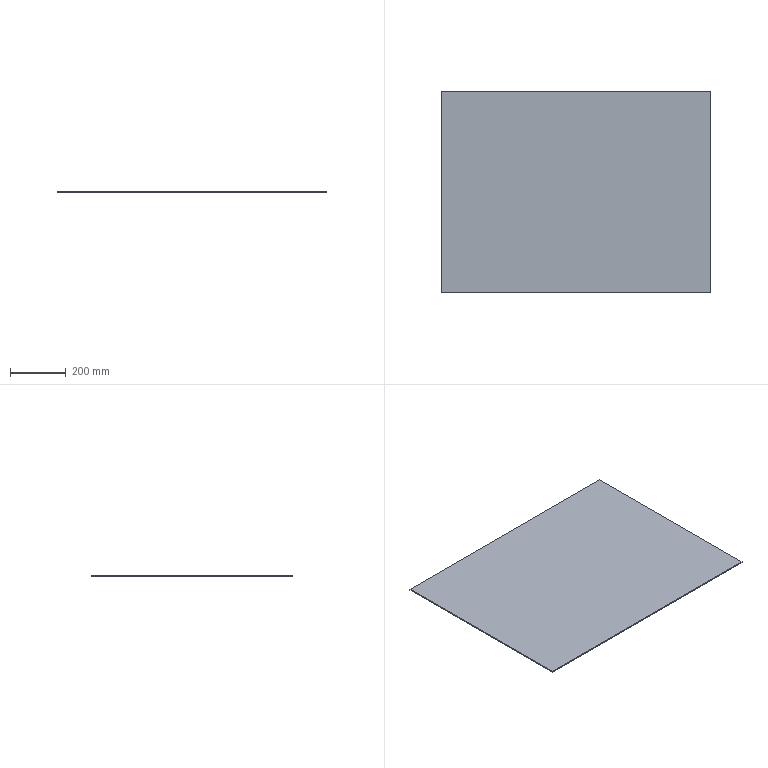Part | STEP file | X77-05501 | 1 solid | 6 faces | box 960 x 720 x 4 mm | volume 2764800 mm3 | plane 6
STEP:
#1=CARTESIAN_POINT('',(521.386,-150.547,0.));
#2=VERTEX_POINT('',#1);
#3=CARTESIAN_POINT('',(521.386,-870.547,0.));
#4=VERTEX_POINT('',#3);
#5=CARTESIAN_POINT('',(521.386,-870.547,0.));
#6=DIRECTION('',(0.,-1.,0.));
#7=VECTOR('',#6,1000.);
#8=LINE('',#5,#7);
#9=EDGE_CURVE('',#2,#4,#8,.T.);
#10=ORIENTED_EDGE('',*,*,#9,.T.);
#11=CARTESIAN_POINT('',(521.386,-870.547,4.));
#12=VERTEX_POINT('',#11);
#13=CARTESIAN_POINT('',(521.386,-870.547,4.));
#14=DIRECTION('',(0.,0.,-1.));
#15=VECTOR('',#14,1000.);
#16=LINE('',#13,#15);
#17=EDGE_CURVE('',#12,#4,#16,.T.);
#18=ORIENTED_EDGE('',*,*,#17,.F.);
#19=CARTESIAN_POINT('',(521.386,-150.547,4.));
#20=VERTEX_POINT('',#19);
#21=CARTESIAN_POINT('',(521.386,-870.547,4.));
#22=DIRECTION('',(0.,-1.,0.));
#23=VECTOR('',#22,1000.);
#24=LINE('',#21,#23);
#25=EDGE_CURVE('',#20,#12,#24,.T.);
#26=ORIENTED_EDGE('',*,*,#25,.F.);
#27=CARTESIAN_POINT('',(521.386,-150.547,4.));
#28=DIRECTION('',(0.,0.,-1.));
#29=VECTOR('',#28,1000.);
#30=LINE('',#27,#29);
#31=EDGE_CURVE('',#20,#2,#30,.T.);
#32=ORIENTED_EDGE('',*,*,#31,.T.);
#33=EDGE_LOOP('',(#10,#18,#26,#32));
#34=FACE_OUTER_BOUND('',#33,.T.);
#35=CARTESIAN_POINT('',(521.386,-870.547,4.));
#36=DIRECTION('',(1.,0.,0.));
#37=DIRECTION('',(0.,0.,-1.));
#38=AXIS2_PLACEMENT_3D('',#35,#36,#37);
#39=PLANE('',#38);
#40=ADVANCED_FACE('',(#34),#39,.F.);
#41=CARTESIAN_POINT('',(1481.386,-870.547,0.));
#42=VERTEX_POINT('',#41);
#43=CARTESIAN_POINT('',(521.386,-870.547,0.));
#44=DIRECTION('',(1.,0.,0.));
#45=VECTOR('',#44,1000.);
#46=LINE('',#43,#45);
#47=EDGE_CURVE('',#4,#42,#46,.T.);
#48=ORIENTED_EDGE('',*,*,#47,.T.);
#49=CARTESIAN_POINT('',(1481.386,-870.547,4.));
#50=VERTEX_POINT('',#49);
#51=CARTESIAN_POINT('',(1481.386,-870.547,4.));
#52=DIRECTION('',(0.,0.,-1.));
#53=VECTOR('',#52,1000.);
#54=LINE('',#51,#53);
#55=EDGE_CURVE('',#50,#42,#54,.T.);
#56=ORIENTED_EDGE('',*,*,#55,.F.);
#57=CARTESIAN_POINT('',(521.386,-870.547,4.));
#58=DIRECTION('',(1.,0.,0.));
#59=VECTOR('',#58,1000.);
#60=LINE('',#57,#59);
#61=EDGE_CURVE('',#12,#50,#60,.T.);
#62=ORIENTED_EDGE('',*,*,#61,.F.);
#63=ORIENTED_EDGE('',*,*,#17,.T.);
#64=EDGE_LOOP('',(#48,#56,#62,#63));
#65=FACE_OUTER_BOUND('',#64,.T.);
#66=CARTESIAN_POINT('',(521.386,-870.547,4.));
#67=DIRECTION('',(0.,1.,0.));
#68=DIRECTION('',(0.,0.,1.));
#69=AXIS2_PLACEMENT_3D('',#66,#67,#68);
#70=PLANE('',#69);
#71=ADVANCED_FACE('',(#65),#70,.F.);
#72=CARTESIAN_POINT('',(1481.386,-150.547,0.));
#73=VERTEX_POINT('',#72);
#74=CARTESIAN_POINT('',(1481.386,-870.547,0.));
#75=DIRECTION('',(0.,1.,0.));
#76=VECTOR('',#75,1000.);
#77=LINE('',#74,#76);
#78=EDGE_CURVE('',#42,#73,#77,.T.);
#79=ORIENTED_EDGE('',*,*,#78,.T.);
#80=CARTESIAN_POINT('',(1481.386,-150.547,4.));
#81=VERTEX_POINT('',#80);
#82=CARTESIAN_POINT('',(1481.386,-150.547,4.));
#83=DIRECTION('',(0.,0.,-1.));
#84=VECTOR('',#83,1000.);
#85=LINE('',#82,#84);
#86=EDGE_CURVE('',#81,#73,#85,.T.);
#87=ORIENTED_EDGE('',*,*,#86,.F.);
#88=CARTESIAN_POINT('',(1481.386,-870.547,4.));
#89=DIRECTION('',(0.,1.,0.));
#90=VECTOR('',#89,1000.);
#91=LINE('',#88,#90);
#92=EDGE_CURVE('',#50,#81,#91,.T.);
#93=ORIENTED_EDGE('',*,*,#92,.F.);
#94=ORIENTED_EDGE('',*,*,#55,.T.);
#95=EDGE_LOOP('',(#79,#87,#93,#94));
#96=FACE_OUTER_BOUND('',#95,.T.);
#97=CARTESIAN_POINT('',(1481.386,-870.547,4.));
#98=DIRECTION('',(-1.,0.,0.));
#99=DIRECTION('',(0.,0.,1.));
#100=AXIS2_PLACEMENT_3D('',#97,#98,#99);
#101=PLANE('',#100);
#102=ADVANCED_FACE('',(#96),#101,.F.);
#103=CARTESIAN_POINT('',(521.386,-150.547,0.));
#104=DIRECTION('',(-1.,0.,0.));
#105=VECTOR('',#104,1000.);
#106=LINE('',#103,#105);
#107=EDGE_CURVE('',#73,#2,#106,.T.);
#108=ORIENTED_EDGE('',*,*,#107,.T.);
#109=ORIENTED_EDGE('',*,*,#31,.F.);
#110=CARTESIAN_POINT('',(521.386,-150.547,4.));
#111=DIRECTION('',(-1.,0.,0.));
#112=VECTOR('',#111,1000.);
#113=LINE('',#110,#112);
#114=EDGE_CURVE('',#81,#20,#113,.T.);
#115=ORIENTED_EDGE('',*,*,#114,.F.);
#116=ORIENTED_EDGE('',*,*,#86,.T.);
#117=EDGE_LOOP('',(#108,#109,#115,#116));
#118=FACE_OUTER_BOUND('',#117,.T.);
#119=CARTESIAN_POINT('',(521.386,-150.547,4.));
#120=DIRECTION('',(0.,-1.,0.));
#121=DIRECTION('',(0.,0.,-1.));
#122=AXIS2_PLACEMENT_3D('',#119,#120,#121);
#123=PLANE('',#122);
#124=ADVANCED_FACE('',(#118),#123,.F.);
#125=ORIENTED_EDGE('',*,*,#25,.T.);
#126=ORIENTED_EDGE('',*,*,#61,.T.);
#127=ORIENTED_EDGE('',*,*,#92,.T.);
#128=ORIENTED_EDGE('',*,*,#114,.T.);
#129=EDGE_LOOP('',(#125,#126,#127,#128));
#130=FACE_OUTER_BOUND('',#129,.T.);
#131=CARTESIAN_POINT('',(521.386,-150.547,4.));
#132=DIRECTION('',(0.,0.,-1.));
#133=DIRECTION('',(-1.,0.,0.));
#134=AXIS2_PLACEMENT_3D('',#131,#132,#133);
#135=PLANE('',#134);
#136=ADVANCED_FACE('',(#130),#135,.F.);
#137=ORIENTED_EDGE('',*,*,#9,.F.);
#138=ORIENTED_EDGE('',*,*,#107,.F.);
#139=ORIENTED_EDGE('',*,*,#78,.F.);
#140=ORIENTED_EDGE('',*,*,#47,.F.);
#141=EDGE_LOOP('',(#137,#138,#139,#140));
#142=FACE_OUTER_BOUND('',#141,.T.);
#143=CARTESIAN_POINT('',(521.386,-150.547,0.));
#144=DIRECTION('',(0.,0.,-1.));
#145=DIRECTION('',(-1.,0.,0.));
#146=AXIS2_PLACEMENT_3D('',#143,#144,#145);
#147=PLANE('',#146);
#148=ADVANCED_FACE('',(#142),#147,.T.);
#149=CLOSED_SHELL('',(#40,#71,#102,#124,#136,#148));
#150=MANIFOLD_SOLID_BREP('',#149);
#151=CARTESIAN_POINT('',(0.,0.,0.));
#152=DIRECTION('',(0.,0.,1.));
#153=DIRECTION('',(1.,0.,0.));
#154=AXIS2_PLACEMENT_3D('',#151,#152,#153);
#155=(LENGTH_UNIT()NAMED_UNIT(*)SI_UNIT(.MILLI.,.METRE.));
#156=UNCERTAINTY_MEASURE_WITH_UNIT(LENGTH_MEASURE(0.00001),#155,'','');
#157=(NAMED_UNIT(*)PLANE_ANGLE_UNIT()SI_UNIT($,.RADIAN.));
#158=(NAMED_UNIT(*)SI_UNIT($,.STERADIAN.)SOLID_ANGLE_UNIT());
#159=(GEOMETRIC_REPRESENTATION_CONTEXT(3)GLOBAL_UNCERTAINTY_ASSIGNED_CONTEXT((#156))GLOBAL_UNIT_ASSIGNED_CONTEXT((#155,#157,#158))REPRESENTATION_CONTEXT('',''));
#160=ADVANCED_BREP_SHAPE_REPRESENTATION('',(#150,#154),#159);